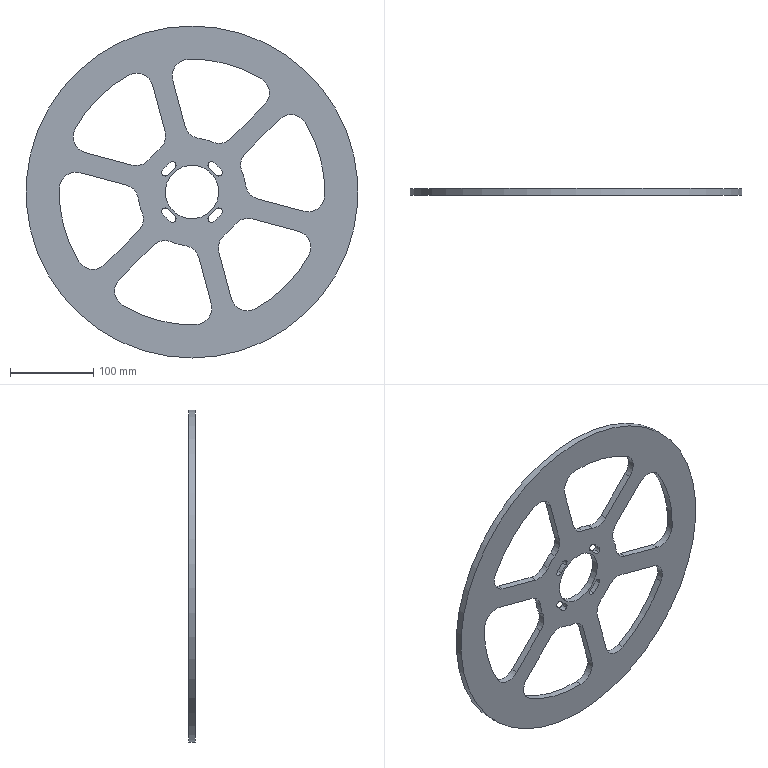Part | STEP file | YBQDJ-FLJ-1 | 1 solid | 76 faces | box 400 x 8 x 400 mm | volume 566908 mm3 | cylinder 62 | plane 14 | commonest cylinder face diameters 40 x24 8.7 x16 130 x6 320 x6 71.3 x4 88.7 x4